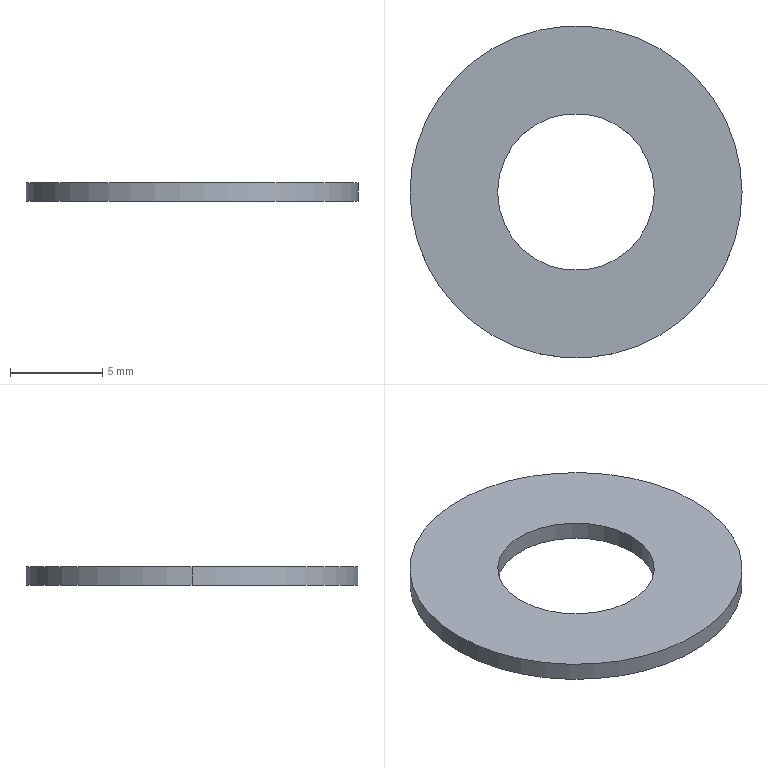Part | SolidWorks | features BaseBody 1 | 1 solid | 6 faces | box 18 x 18 x 1 mm | volume 197.724 mm3 | cylinder 4 | plane 2 | commonest cylinder face diameters 8.5 x2 18 x2
STEP:
#1=CARTESIAN_POINT('',(4.25,0.,1.));
#2=VERTEX_POINT('',#1);
#3=CARTESIAN_POINT('',(-4.25,0.,1.));
#4=VERTEX_POINT('',#3);
#5=CARTESIAN_POINT('',(0.,0.,1.));
#6=DIRECTION('',(0.,0.,-1.));
#7=DIRECTION('',(-1.,0.,0.));
#8=AXIS2_PLACEMENT_3D('',#5,#6,#7);
#9=CIRCLE('',#8,4.25);
#10=EDGE_CURVE('',#2,#4,#9,.T.);
#11=ORIENTED_EDGE('',*,*,#10,.F.);
#12=CARTESIAN_POINT('',(4.25,0.,0.));
#13=VERTEX_POINT('',#12);
#14=CARTESIAN_POINT('',(4.25,0.,1.));
#15=DIRECTION('',(0.,0.,-1.));
#16=VECTOR('',#15,1000.);
#17=LINE('',#14,#16);
#18=EDGE_CURVE('',#2,#13,#17,.T.);
#19=ORIENTED_EDGE('',*,*,#18,.T.);
#20=CARTESIAN_POINT('',(-4.25,0.,0.));
#21=VERTEX_POINT('',#20);
#22=CARTESIAN_POINT('',(0.,0.,0.));
#23=DIRECTION('',(0.,0.,1.));
#24=DIRECTION('',(-1.,0.,0.));
#25=AXIS2_PLACEMENT_3D('',#22,#23,#24);
#26=CIRCLE('',#25,4.25);
#27=EDGE_CURVE('',#21,#13,#26,.T.);
#28=ORIENTED_EDGE('',*,*,#27,.F.);
#29=CARTESIAN_POINT('',(-4.25,0.,1.));
#30=DIRECTION('',(0.,0.,-1.));
#31=VECTOR('',#30,1000.);
#32=LINE('',#29,#31);
#33=EDGE_CURVE('',#4,#21,#32,.T.);
#34=ORIENTED_EDGE('',*,*,#33,.F.);
#35=EDGE_LOOP('',(#11,#19,#28,#34));
#36=FACE_OUTER_BOUND('',#35,.T.);
#37=CARTESIAN_POINT('',(0.,0.,1.));
#38=DIRECTION('',(0.,0.,-1.));
#39=DIRECTION('',(-1.,0.,0.));
#40=AXIS2_PLACEMENT_3D('',#37,#38,#39);
#41=CYLINDRICAL_SURFACE('',#40,4.25);
#42=ADVANCED_FACE('',(#36),#41,.F.);
#43=CARTESIAN_POINT('',(9.,0.,1.));
#44=VERTEX_POINT('',#43);
#45=CARTESIAN_POINT('',(-9.,0.,1.));
#46=VERTEX_POINT('',#45);
#47=CARTESIAN_POINT('',(0.,0.,1.));
#48=DIRECTION('',(0.,0.,1.));
#49=DIRECTION('',(-1.,0.,0.));
#50=AXIS2_PLACEMENT_3D('',#47,#48,#49);
#51=CIRCLE('',#50,9.);
#52=EDGE_CURVE('',#44,#46,#51,.T.);
#53=ORIENTED_EDGE('',*,*,#52,.F.);
#54=CARTESIAN_POINT('',(9.,0.,0.));
#55=VERTEX_POINT('',#54);
#56=CARTESIAN_POINT('',(9.,0.,1.));
#57=DIRECTION('',(0.,0.,-1.));
#58=VECTOR('',#57,1000.);
#59=LINE('',#56,#58);
#60=EDGE_CURVE('',#44,#55,#59,.T.);
#61=ORIENTED_EDGE('',*,*,#60,.T.);
#62=CARTESIAN_POINT('',(-9.,0.,0.));
#63=VERTEX_POINT('',#62);
#64=CARTESIAN_POINT('',(0.,0.,0.));
#65=DIRECTION('',(0.,0.,1.));
#66=DIRECTION('',(-1.,0.,0.));
#67=AXIS2_PLACEMENT_3D('',#64,#65,#66);
#68=CIRCLE('',#67,9.);
#69=EDGE_CURVE('',#55,#63,#68,.T.);
#70=ORIENTED_EDGE('',*,*,#69,.T.);
#71=CARTESIAN_POINT('',(-9.,0.,1.));
#72=DIRECTION('',(0.,0.,-1.));
#73=VECTOR('',#72,1000.);
#74=LINE('',#71,#73);
#75=EDGE_CURVE('',#46,#63,#74,.T.);
#76=ORIENTED_EDGE('',*,*,#75,.F.);
#77=EDGE_LOOP('',(#53,#61,#70,#76));
#78=FACE_OUTER_BOUND('',#77,.T.);
#79=CARTESIAN_POINT('',(0.,0.,1.));
#80=DIRECTION('',(0.,0.,-1.));
#81=DIRECTION('',(-1.,0.,0.));
#82=AXIS2_PLACEMENT_3D('',#79,#80,#81);
#83=CYLINDRICAL_SURFACE('',#82,9.);
#84=ADVANCED_FACE('',(#78),#83,.T.);
#85=CARTESIAN_POINT('',(0.,0.,1.));
#86=DIRECTION('',(0.,0.,-1.));
#87=DIRECTION('',(-1.,0.,0.));
#88=AXIS2_PLACEMENT_3D('',#85,#86,#87);
#89=CIRCLE('',#88,4.25);
#90=EDGE_CURVE('',#4,#2,#89,.T.);
#91=ORIENTED_EDGE('',*,*,#90,.T.);
#92=ORIENTED_EDGE('',*,*,#10,.T.);
#93=EDGE_LOOP('',(#91,#92));
#94=FACE_BOUND('',#93,.T.);
#95=CARTESIAN_POINT('',(0.,0.,1.));
#96=DIRECTION('',(0.,0.,1.));
#97=DIRECTION('',(-1.,0.,0.));
#98=AXIS2_PLACEMENT_3D('',#95,#96,#97);
#99=CIRCLE('',#98,9.);
#100=EDGE_CURVE('',#46,#44,#99,.T.);
#101=ORIENTED_EDGE('',*,*,#100,.T.);
#102=ORIENTED_EDGE('',*,*,#52,.T.);
#103=EDGE_LOOP('',(#101,#102));
#104=FACE_OUTER_BOUND('',#103,.T.);
#105=CARTESIAN_POINT('',(0.,0.,1.));
#106=DIRECTION('',(0.,0.,1.));
#107=DIRECTION('',(1.,0.,0.));
#108=AXIS2_PLACEMENT_3D('',#105,#106,#107);
#109=PLANE('',#108);
#110=ADVANCED_FACE('',(#94,#104),#109,.T.);
#111=ORIENTED_EDGE('',*,*,#18,.F.);
#112=ORIENTED_EDGE('',*,*,#90,.F.);
#113=ORIENTED_EDGE('',*,*,#33,.T.);
#114=CARTESIAN_POINT('',(0.,0.,0.));
#115=DIRECTION('',(0.,0.,1.));
#116=DIRECTION('',(-1.,0.,0.));
#117=AXIS2_PLACEMENT_3D('',#114,#115,#116);
#118=CIRCLE('',#117,4.25);
#119=EDGE_CURVE('',#13,#21,#118,.T.);
#120=ORIENTED_EDGE('',*,*,#119,.F.);
#121=EDGE_LOOP('',(#111,#112,#113,#120));
#122=FACE_OUTER_BOUND('',#121,.T.);
#123=CARTESIAN_POINT('',(0.,0.,1.));
#124=DIRECTION('',(0.,0.,-1.));
#125=DIRECTION('',(-1.,0.,0.));
#126=AXIS2_PLACEMENT_3D('',#123,#124,#125);
#127=CYLINDRICAL_SURFACE('',#126,4.25);
#128=ADVANCED_FACE('',(#122),#127,.F.);
#129=ORIENTED_EDGE('',*,*,#60,.F.);
#130=ORIENTED_EDGE('',*,*,#100,.F.);
#131=ORIENTED_EDGE('',*,*,#75,.T.);
#132=CARTESIAN_POINT('',(0.,0.,0.));
#133=DIRECTION('',(0.,0.,1.));
#134=DIRECTION('',(-1.,0.,0.));
#135=AXIS2_PLACEMENT_3D('',#132,#133,#134);
#136=CIRCLE('',#135,9.);
#137=EDGE_CURVE('',#63,#55,#136,.T.);
#138=ORIENTED_EDGE('',*,*,#137,.T.);
#139=EDGE_LOOP('',(#129,#130,#131,#138));
#140=FACE_OUTER_BOUND('',#139,.T.);
#141=CARTESIAN_POINT('',(0.,0.,1.));
#142=DIRECTION('',(0.,0.,-1.));
#143=DIRECTION('',(-1.,0.,0.));
#144=AXIS2_PLACEMENT_3D('',#141,#142,#143);
#145=CYLINDRICAL_SURFACE('',#144,9.);
#146=ADVANCED_FACE('',(#140),#145,.T.);
#147=ORIENTED_EDGE('',*,*,#27,.T.);
#148=ORIENTED_EDGE('',*,*,#119,.T.);
#149=EDGE_LOOP('',(#147,#148));
#150=FACE_BOUND('',#149,.T.);
#151=ORIENTED_EDGE('',*,*,#137,.F.);
#152=ORIENTED_EDGE('',*,*,#69,.F.);
#153=EDGE_LOOP('',(#151,#152));
#154=FACE_OUTER_BOUND('',#153,.T.);
#155=CARTESIAN_POINT('',(0.,0.,0.));
#156=DIRECTION('',(0.,0.,1.));
#157=DIRECTION('',(1.,0.,0.));
#158=AXIS2_PLACEMENT_3D('',#155,#156,#157);
#159=PLANE('',#158);
#160=ADVANCED_FACE('',(#150,#154),#159,.F.);
#161=CLOSED_SHELL('',(#42,#84,#110,#128,#146,#160));
#162=MANIFOLD_SOLID_BREP('',#161);
#163=CARTESIAN_POINT('',(0.,0.,0.));
#164=DIRECTION('',(0.,0.,1.));
#165=DIRECTION('',(1.,0.,0.));
#166=AXIS2_PLACEMENT_3D('',#163,#164,#165);
#167=(LENGTH_UNIT()NAMED_UNIT(*)SI_UNIT(.MILLI.,.METRE.));
#168=UNCERTAINTY_MEASURE_WITH_UNIT(LENGTH_MEASURE(0.00001),#167,'','');
#169=(NAMED_UNIT(*)PLANE_ANGLE_UNIT()SI_UNIT($,.RADIAN.));
#170=(NAMED_UNIT(*)SI_UNIT($,.STERADIAN.)SOLID_ANGLE_UNIT());
#171=(GEOMETRIC_REPRESENTATION_CONTEXT(3)GLOBAL_UNCERTAINTY_ASSIGNED_CONTEXT((#168))GLOBAL_UNIT_ASSIGNED_CONTEXT((#167,#169,#170))REPRESENTATION_CONTEXT('',''));
#172=ADVANCED_BREP_SHAPE_REPRESENTATION('',(#162,#166),#171);